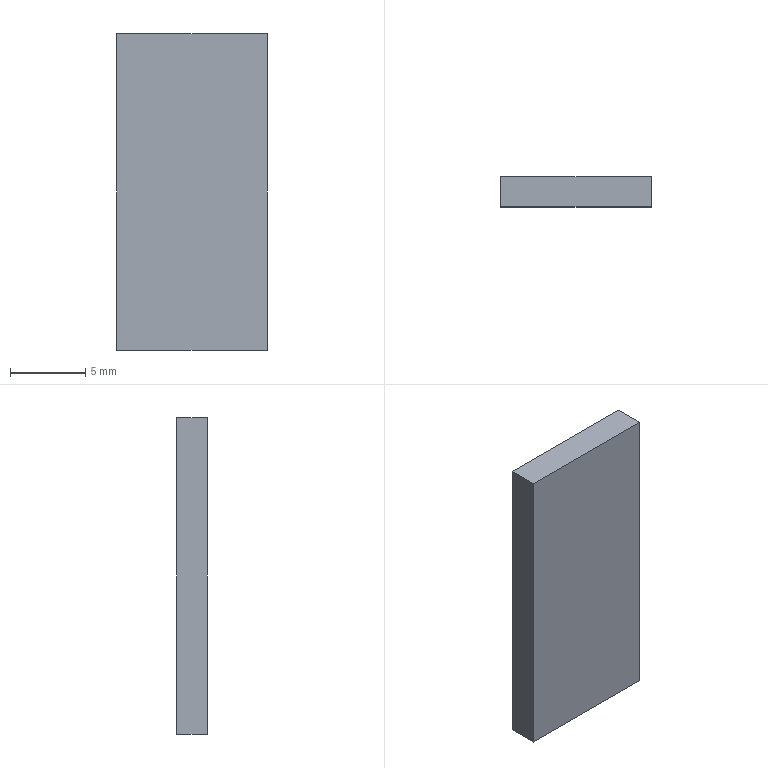Part | SolidWorks | features BaseBody 1 | 1 solid | 6 faces | box 10 x 2 x 21 mm | volume 420 mm3 | plane 6
STEP:
#1=CARTESIAN_POINT('',(10.,0.,-21.));
#2=VERTEX_POINT('',#1);
#3=CARTESIAN_POINT('',(0.,0.,-21.));
#4=VERTEX_POINT('',#3);
#5=CARTESIAN_POINT('',(0.,0.,-21.));
#6=DIRECTION('',(-1.,0.,0.));
#7=VECTOR('',#6,1000.);
#8=LINE('',#5,#7);
#9=EDGE_CURVE('',#2,#4,#8,.T.);
#10=ORIENTED_EDGE('',*,*,#9,.F.);
#11=CARTESIAN_POINT('',(10.,0.,0.));
#12=VERTEX_POINT('',#11);
#13=CARTESIAN_POINT('',(10.,0.,0.));
#14=DIRECTION('',(0.,0.,-1.));
#15=VECTOR('',#14,1000.);
#16=LINE('',#13,#15);
#17=EDGE_CURVE('',#12,#2,#16,.T.);
#18=ORIENTED_EDGE('',*,*,#17,.F.);
#19=CARTESIAN_POINT('',(0.,0.,0.));
#20=VERTEX_POINT('',#19);
#21=CARTESIAN_POINT('',(0.,0.,0.));
#22=DIRECTION('',(1.,0.,0.));
#23=VECTOR('',#22,1000.);
#24=LINE('',#21,#23);
#25=EDGE_CURVE('',#20,#12,#24,.T.);
#26=ORIENTED_EDGE('',*,*,#25,.F.);
#27=CARTESIAN_POINT('',(0.,0.,0.));
#28=DIRECTION('',(0.,0.,1.));
#29=VECTOR('',#28,1000.);
#30=LINE('',#27,#29);
#31=EDGE_CURVE('',#4,#20,#30,.T.);
#32=ORIENTED_EDGE('',*,*,#31,.F.);
#33=EDGE_LOOP('',(#10,#18,#26,#32));
#34=FACE_OUTER_BOUND('',#33,.T.);
#35=CARTESIAN_POINT('',(0.,0.,0.));
#36=DIRECTION('',(0.,1.,0.));
#37=DIRECTION('',(0.,0.,1.));
#38=AXIS2_PLACEMENT_3D('',#35,#36,#37);
#39=PLANE('',#38);
#40=ADVANCED_FACE('',(#34),#39,.F.);
#41=CARTESIAN_POINT('',(0.,2.,-21.));
#42=VERTEX_POINT('',#41);
#43=CARTESIAN_POINT('',(0.,0.,-21.));
#44=DIRECTION('',(0.,-1.,0.));
#45=VECTOR('',#44,1000.);
#46=LINE('',#43,#45);
#47=EDGE_CURVE('',#42,#4,#46,.T.);
#48=ORIENTED_EDGE('',*,*,#47,.T.);
#49=ORIENTED_EDGE('',*,*,#31,.T.);
#50=CARTESIAN_POINT('',(0.,2.,0.));
#51=VERTEX_POINT('',#50);
#52=CARTESIAN_POINT('',(0.,0.,0.));
#53=DIRECTION('',(0.,1.,0.));
#54=VECTOR('',#53,1000.);
#55=LINE('',#52,#54);
#56=EDGE_CURVE('',#20,#51,#55,.T.);
#57=ORIENTED_EDGE('',*,*,#56,.T.);
#58=CARTESIAN_POINT('',(0.,2.,-21.));
#59=DIRECTION('',(0.,0.,-1.));
#60=VECTOR('',#59,1000.);
#61=LINE('',#58,#60);
#62=EDGE_CURVE('',#51,#42,#61,.T.);
#63=ORIENTED_EDGE('',*,*,#62,.T.);
#64=EDGE_LOOP('',(#48,#49,#57,#63));
#65=FACE_OUTER_BOUND('',#64,.T.);
#66=CARTESIAN_POINT('',(0.,0.,-21.));
#67=DIRECTION('',(-1.,0.,0.));
#68=DIRECTION('',(0.,0.,1.));
#69=AXIS2_PLACEMENT_3D('',#66,#67,#68);
#70=PLANE('',#69);
#71=ADVANCED_FACE('',(#65),#70,.T.);
#72=CARTESIAN_POINT('',(10.,2.,-21.));
#73=VERTEX_POINT('',#72);
#74=CARTESIAN_POINT('',(10.,0.,-21.));
#75=DIRECTION('',(0.,-1.,0.));
#76=VECTOR('',#75,1000.);
#77=LINE('',#74,#76);
#78=EDGE_CURVE('',#73,#2,#77,.T.);
#79=ORIENTED_EDGE('',*,*,#78,.T.);
#80=ORIENTED_EDGE('',*,*,#9,.T.);
#81=ORIENTED_EDGE('',*,*,#47,.F.);
#82=CARTESIAN_POINT('',(10.,2.,-21.));
#83=DIRECTION('',(1.,0.,0.));
#84=VECTOR('',#83,1000.);
#85=LINE('',#82,#84);
#86=EDGE_CURVE('',#42,#73,#85,.T.);
#87=ORIENTED_EDGE('',*,*,#86,.T.);
#88=EDGE_LOOP('',(#79,#80,#81,#87));
#89=FACE_OUTER_BOUND('',#88,.T.);
#90=CARTESIAN_POINT('',(10.,0.,-21.));
#91=DIRECTION('',(0.,0.,-1.));
#92=DIRECTION('',(-1.,0.,0.));
#93=AXIS2_PLACEMENT_3D('',#90,#91,#92);
#94=PLANE('',#93);
#95=ADVANCED_FACE('',(#89),#94,.T.);
#96=CARTESIAN_POINT('',(10.,2.,0.));
#97=VERTEX_POINT('',#96);
#98=CARTESIAN_POINT('',(10.,0.,0.));
#99=DIRECTION('',(0.,-1.,0.));
#100=VECTOR('',#99,1000.);
#101=LINE('',#98,#100);
#102=EDGE_CURVE('',#97,#12,#101,.T.);
#103=ORIENTED_EDGE('',*,*,#102,.T.);
#104=ORIENTED_EDGE('',*,*,#17,.T.);
#105=ORIENTED_EDGE('',*,*,#78,.F.);
#106=CARTESIAN_POINT('',(10.,2.,0.));
#107=DIRECTION('',(0.,0.,1.));
#108=VECTOR('',#107,1000.);
#109=LINE('',#106,#108);
#110=EDGE_CURVE('',#73,#97,#109,.T.);
#111=ORIENTED_EDGE('',*,*,#110,.T.);
#112=EDGE_LOOP('',(#103,#104,#105,#111));
#113=FACE_OUTER_BOUND('',#112,.T.);
#114=CARTESIAN_POINT('',(10.,0.,0.));
#115=DIRECTION('',(1.,0.,0.));
#116=DIRECTION('',(0.,0.,-1.));
#117=AXIS2_PLACEMENT_3D('',#114,#115,#116);
#118=PLANE('',#117);
#119=ADVANCED_FACE('',(#113),#118,.T.);
#120=ORIENTED_EDGE('',*,*,#56,.F.);
#121=ORIENTED_EDGE('',*,*,#25,.T.);
#122=ORIENTED_EDGE('',*,*,#102,.F.);
#123=CARTESIAN_POINT('',(0.,2.,0.));
#124=DIRECTION('',(-1.,0.,0.));
#125=VECTOR('',#124,1000.);
#126=LINE('',#123,#125);
#127=EDGE_CURVE('',#97,#51,#126,.T.);
#128=ORIENTED_EDGE('',*,*,#127,.T.);
#129=EDGE_LOOP('',(#120,#121,#122,#128));
#130=FACE_OUTER_BOUND('',#129,.T.);
#131=CARTESIAN_POINT('',(0.,0.,0.));
#132=DIRECTION('',(0.,0.,1.));
#133=DIRECTION('',(1.,0.,0.));
#134=AXIS2_PLACEMENT_3D('',#131,#132,#133);
#135=PLANE('',#134);
#136=ADVANCED_FACE('',(#130),#135,.T.);
#137=ORIENTED_EDGE('',*,*,#62,.F.);
#138=ORIENTED_EDGE('',*,*,#127,.F.);
#139=ORIENTED_EDGE('',*,*,#110,.F.);
#140=ORIENTED_EDGE('',*,*,#86,.F.);
#141=EDGE_LOOP('',(#137,#138,#139,#140));
#142=FACE_OUTER_BOUND('',#141,.T.);
#143=CARTESIAN_POINT('',(0.,2.,0.));
#144=DIRECTION('',(0.,1.,0.));
#145=DIRECTION('',(0.,0.,1.));
#146=AXIS2_PLACEMENT_3D('',#143,#144,#145);
#147=PLANE('',#146);
#148=ADVANCED_FACE('',(#142),#147,.T.);
#149=CLOSED_SHELL('',(#40,#71,#95,#119,#136,#148));
#150=MANIFOLD_SOLID_BREP('',#149);
#151=CARTESIAN_POINT('',(0.,0.,0.));
#152=DIRECTION('',(0.,0.,1.));
#153=DIRECTION('',(1.,0.,0.));
#154=AXIS2_PLACEMENT_3D('',#151,#152,#153);
#155=(LENGTH_UNIT()NAMED_UNIT(*)SI_UNIT(.MILLI.,.METRE.));
#156=UNCERTAINTY_MEASURE_WITH_UNIT(LENGTH_MEASURE(0.00001),#155,'','');
#157=(NAMED_UNIT(*)PLANE_ANGLE_UNIT()SI_UNIT($,.RADIAN.));
#158=(NAMED_UNIT(*)SI_UNIT($,.STERADIAN.)SOLID_ANGLE_UNIT());
#159=(GEOMETRIC_REPRESENTATION_CONTEXT(3)GLOBAL_UNCERTAINTY_ASSIGNED_CONTEXT((#156))GLOBAL_UNIT_ASSIGNED_CONTEXT((#155,#157,#158))REPRESENTATION_CONTEXT('',''));
#160=ADVANCED_BREP_SHAPE_REPRESENTATION('',(#150,#154),#159);